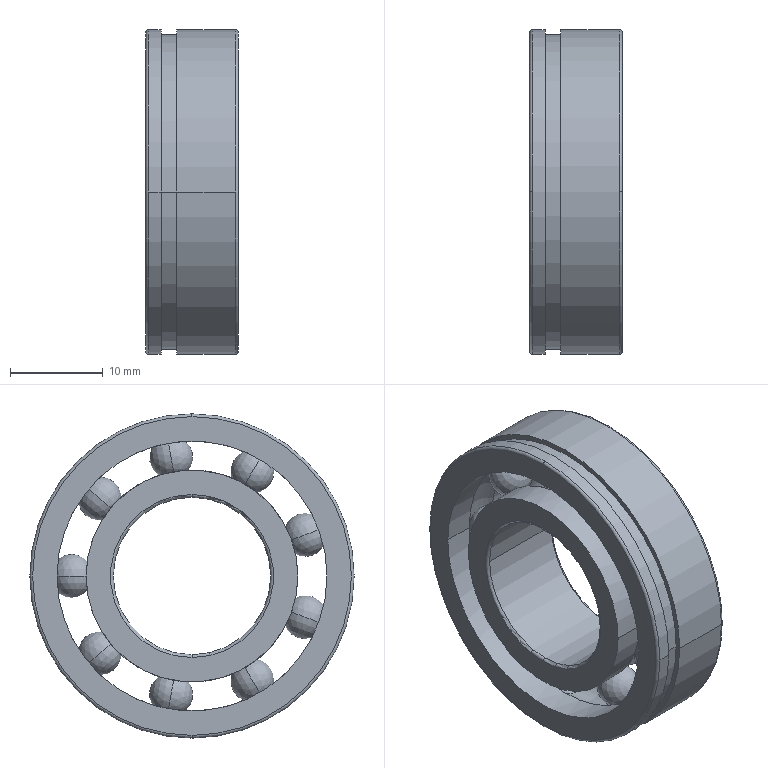Part | SolidWorks | features BaseBody 11 | 11 solids | 54 faces | box 10 x 35 x 35 mm | volume 4868 mm3 | sphere 18 | cylinder 16 | torus 14 | plane 6 | commonest cylinder face diameters 22.868 x4 29.132 x4 35 x4 17 x2 33.92 x2
STEP:
#1=CARTESIAN_POINT('',(5.,10.66,0.));
#2=VERTEX_POINT('',#1);
#3=CARTESIAN_POINT('',(5.,15.34,0.));
#4=VERTEX_POINT('',#3);
#5=CARTESIAN_POINT('',(5.,13.,0.));
#6=DIRECTION('',(0.,0.,1.));
#7=DIRECTION('',(1.,0.,0.));
#8=AXIS2_PLACEMENT_3D('',#5,#6,#7);
#9=CIRCLE('',#8,2.34);
#10=EDGE_CURVE('',#2,#4,#9,.T.);
#11=ORIENTED_EDGE('',*,*,#10,.F.);
#12=CARTESIAN_POINT('',(5.,13.,0.));
#13=DIRECTION('',(0.,0.,-1.));
#14=DIRECTION('',(-1.,0.,0.));
#15=AXIS2_PLACEMENT_3D('',#12,#13,#14);
#16=CIRCLE('',#15,2.34);
#17=EDGE_CURVE('',#2,#4,#16,.T.);
#18=ORIENTED_EDGE('',*,*,#17,.T.);
#19=EDGE_LOOP('',(#11,#18));
#20=FACE_OUTER_BOUND('',#19,.T.);
#21=CARTESIAN_POINT('',(5.,13.,0.));
#22=DIRECTION('',(0.,0.,-1.));
#23=DIRECTION('',(1.,0.,0.));
#24=AXIS2_PLACEMENT_3D('',#21,#22,#23);
#25=SPHERICAL_SURFACE('',#24,2.34);
#26=ADVANCED_FACE('',(#20),#25,.T.);
#27=ORIENTED_EDGE('',*,*,#17,.F.);
#28=ORIENTED_EDGE('',*,*,#10,.T.);
#29=EDGE_LOOP('',(#27,#28));
#30=FACE_OUTER_BOUND('',#29,.T.);
#31=CARTESIAN_POINT('',(5.,13.,0.));
#32=DIRECTION('',(0.,0.,-1.));
#33=DIRECTION('',(1.,0.,0.));
#34=AXIS2_PLACEMENT_3D('',#31,#32,#33);
#35=SPHERICAL_SURFACE('',#34,2.34);
#36=ADVANCED_FACE('',(#30),#35,.T.);
#37=CLOSED_SHELL('',(#26,#36));
#38=MANIFOLD_SOLID_BREP('',#37);
#39=CARTESIAN_POINT('',(3.333,-16.96,0.));
#40=VERTEX_POINT('',#39);
#41=CARTESIAN_POINT('',(3.333,16.96,0.));
#42=VERTEX_POINT('',#41);
#43=CARTESIAN_POINT('',(3.333,0.,0.));
#44=DIRECTION('',(1.,0.,0.));
#45=DIRECTION('',(0.,1.,0.));
#46=AXIS2_PLACEMENT_3D('',#43,#44,#45);
#47=CIRCLE('',#46,16.96);
#48=EDGE_CURVE('',#40,#42,#47,.T.);
#49=ORIENTED_EDGE('',*,*,#48,.F.);
#50=CARTESIAN_POINT('',(1.667,-16.96,0.));
#51=VERTEX_POINT('',#50);
#52=CARTESIAN_POINT('',(2.5,-16.96,0.));
#53=DIRECTION('',(-1.,0.,0.));
#54=VECTOR('',#53,1000.);
#55=LINE('',#52,#54);
#56=EDGE_CURVE('',#40,#51,#55,.T.);
#57=ORIENTED_EDGE('',*,*,#56,.T.);
#58=CARTESIAN_POINT('',(1.667,16.96,0.));
#59=VERTEX_POINT('',#58);
#60=CARTESIAN_POINT('',(1.667,0.,0.));
#61=DIRECTION('',(1.,0.,0.));
#62=DIRECTION('',(0.,1.,0.));
#63=AXIS2_PLACEMENT_3D('',#60,#61,#62);
#64=CIRCLE('',#63,16.96);
#65=EDGE_CURVE('',#51,#59,#64,.T.);
#66=ORIENTED_EDGE('',*,*,#65,.T.);
#67=CARTESIAN_POINT('',(2.5,16.96,0.));
#68=DIRECTION('',(-1.,0.,0.));
#69=VECTOR('',#68,1000.);
#70=LINE('',#67,#69);
#71=EDGE_CURVE('',#42,#59,#70,.T.);
#72=ORIENTED_EDGE('',*,*,#71,.F.);
#73=EDGE_LOOP('',(#49,#57,#66,#72));
#74=FACE_OUTER_BOUND('',#73,.T.);
#75=CARTESIAN_POINT('',(2.5,0.,0.));
#76=DIRECTION('',(-1.,0.,0.));
#77=DIRECTION('',(0.,1.,0.));
#78=AXIS2_PLACEMENT_3D('',#75,#76,#77);
#79=CYLINDRICAL_SURFACE('',#78,16.96);
#80=ADVANCED_FACE('',(#74),#79,.T.);
#81=CARTESIAN_POINT('',(9.7,-17.5,0.));
#82=VERTEX_POINT('',#81);
#83=CARTESIAN_POINT('',(9.7,0.,-17.5));
#84=VERTEX_POINT('',#83);
#85=CARTESIAN_POINT('',(9.7,0.,0.));
#86=DIRECTION('',(1.,0.,0.));
#87=DIRECTION('',(0.,-1.,0.));
#88=AXIS2_PLACEMENT_3D('',#85,#86,#87);
#89=CIRCLE('',#88,17.5);
#90=EDGE_CURVE('',#82,#84,#89,.T.);
#91=ORIENTED_EDGE('',*,*,#90,.F.);
#92=CARTESIAN_POINT('',(3.333,-17.5,0.));
#93=VERTEX_POINT('',#92);
#94=CARTESIAN_POINT('',(6.667,-17.5,0.));
#95=DIRECTION('',(-1.,0.,0.));
#96=VECTOR('',#95,1000.);
#97=LINE('',#94,#96);
#98=EDGE_CURVE('',#82,#93,#97,.T.);
#99=ORIENTED_EDGE('',*,*,#98,.T.);
#100=CARTESIAN_POINT('',(3.333,17.5,0.));
#101=VERTEX_POINT('',#100);
#102=CARTESIAN_POINT('',(3.333,0.,0.));
#103=DIRECTION('',(1.,0.,0.));
#104=DIRECTION('',(0.,1.,0.));
#105=AXIS2_PLACEMENT_3D('',#102,#103,#104);
#106=CIRCLE('',#105,17.5);
#107=EDGE_CURVE('',#93,#101,#106,.T.);
#108=ORIENTED_EDGE('',*,*,#107,.T.);
#109=CARTESIAN_POINT('',(9.7,17.5,0.));
#110=VERTEX_POINT('',#109);
#111=CARTESIAN_POINT('',(6.667,17.5,0.));
#112=DIRECTION('',(-1.,0.,0.));
#113=VECTOR('',#112,1000.);
#114=LINE('',#111,#113);
#115=EDGE_CURVE('',#110,#101,#114,.T.);
#116=ORIENTED_EDGE('',*,*,#115,.F.);
#117=CARTESIAN_POINT('',(9.7,0.,0.));
#118=DIRECTION('',(1.,0.,0.));
#119=DIRECTION('',(0.,-1.,0.));
#120=AXIS2_PLACEMENT_3D('',#117,#118,#119);
#121=CIRCLE('',#120,17.5);
#122=EDGE_CURVE('',#84,#110,#121,.T.);
#123=ORIENTED_EDGE('',*,*,#122,.F.);
#124=EDGE_LOOP('',(#91,#99,#108,#116,#123));
#125=FACE_OUTER_BOUND('',#124,.T.);
#126=CARTESIAN_POINT('',(6.667,0.,0.));
#127=DIRECTION('',(-1.,0.,0.));
#128=DIRECTION('',(0.,1.,0.));
#129=AXIS2_PLACEMENT_3D('',#126,#127,#128);
#130=CYLINDRICAL_SURFACE('',#129,17.5);
#131=ADVANCED_FACE('',(#125),#130,.T.);
#132=CARTESIAN_POINT('',(1.667,-17.5,0.));
#133=VERTEX_POINT('',#132);
#134=CARTESIAN_POINT('',(1.667,17.5,0.));
#135=VERTEX_POINT('',#134);
#136=CARTESIAN_POINT('',(1.667,0.,0.));
#137=DIRECTION('',(1.,0.,0.));
#138=DIRECTION('',(0.,1.,0.));
#139=AXIS2_PLACEMENT_3D('',#136,#137,#138);
#140=CIRCLE('',#139,17.5);
#141=EDGE_CURVE('',#133,#135,#140,.T.);
#142=ORIENTED_EDGE('',*,*,#141,.F.);
#143=CARTESIAN_POINT('',(0.3,-17.5,0.));
#144=VERTEX_POINT('',#143);
#145=CARTESIAN_POINT('',(0.8333,-17.5,0.));
#146=DIRECTION('',(-1.,0.,0.));
#147=VECTOR('',#146,1000.);
#148=LINE('',#145,#147);
#149=EDGE_CURVE('',#133,#144,#148,.T.);
#150=ORIENTED_EDGE('',*,*,#149,.T.);
#151=CARTESIAN_POINT('',(0.3,0.,-17.5));
#152=VERTEX_POINT('',#151);
#153=CARTESIAN_POINT('',(0.3,0.,0.));
#154=DIRECTION('',(-1.,0.,0.));
#155=DIRECTION('',(0.,-1.,0.));
#156=AXIS2_PLACEMENT_3D('',#153,#154,#155);
#157=CIRCLE('',#156,17.5);
#158=EDGE_CURVE('',#152,#144,#157,.T.);
#159=ORIENTED_EDGE('',*,*,#158,.F.);
#160=CARTESIAN_POINT('',(0.3,17.5,0.));
#161=VERTEX_POINT('',#160);
#162=CARTESIAN_POINT('',(0.3,0.,0.));
#163=DIRECTION('',(-1.,0.,0.));
#164=DIRECTION('',(0.,-1.,0.));
#165=AXIS2_PLACEMENT_3D('',#162,#163,#164);
#166=CIRCLE('',#165,17.5);
#167=EDGE_CURVE('',#161,#152,#166,.T.);
#168=ORIENTED_EDGE('',*,*,#167,.F.);
#169=CARTESIAN_POINT('',(0.8333,17.5,0.));
#170=DIRECTION('',(-1.,0.,0.));
#171=VECTOR('',#170,1000.);
#172=LINE('',#169,#171);
#173=EDGE_CURVE('',#135,#161,#172,.T.);
#174=ORIENTED_EDGE('',*,*,#173,.F.);
#175=EDGE_LOOP('',(#142,#150,#159,#168,#174));
#176=FACE_OUTER_BOUND('',#175,.T.);
#177=CARTESIAN_POINT('',(0.8333,0.,0.));
#178=DIRECTION('',(-1.,0.,0.));
#179=DIRECTION('',(0.,1.,0.));
#180=AXIS2_PLACEMENT_3D('',#177,#178,#179);
#181=CYLINDRICAL_SURFACE('',#180,17.5);
#182=ADVANCED_FACE('',(#176),#181,.T.);
#183=ORIENTED_EDGE('',*,*,#122,.T.);
#184=CARTESIAN_POINT('',(9.7,0.,17.5));
#185=VERTEX_POINT('',#184);
#186=CARTESIAN_POINT('',(9.7,0.,0.));
#187=DIRECTION('',(1.,0.,0.));
#188=DIRECTION('',(0.,-1.,0.));
#189=AXIS2_PLACEMENT_3D('',#186,#187,#188);
#190=CIRCLE('',#189,17.5);
#191=EDGE_CURVE('',#110,#185,#190,.T.);
#192=ORIENTED_EDGE('',*,*,#191,.T.);
#193=CARTESIAN_POINT('',(10.,0.,17.2));
#194=VERTEX_POINT('',#193);
#195=CARTESIAN_POINT('',(9.7,0.,17.2));
#196=DIRECTION('',(0.,1.,0.));
#197=DIRECTION('',(0.,0.,1.));
#198=AXIS2_PLACEMENT_3D('',#195,#196,#197);
#199=CIRCLE('',#198,0.3);
#200=EDGE_CURVE('',#185,#194,#199,.T.);
#201=ORIENTED_EDGE('',*,*,#200,.T.);
#202=CARTESIAN_POINT('',(10.,0.,-17.2));
#203=VERTEX_POINT('',#202);
#204=CARTESIAN_POINT('',(10.,0.,0.));
#205=DIRECTION('',(-1.,0.,0.));
#206=DIRECTION('',(0.,-1.,0.));
#207=AXIS2_PLACEMENT_3D('',#204,#205,#206);
#208=CIRCLE('',#207,17.2);
#209=EDGE_CURVE('',#194,#203,#208,.T.);
#210=ORIENTED_EDGE('',*,*,#209,.T.);
#211=CARTESIAN_POINT('',(9.7,0.,-17.2));
#212=DIRECTION('',(0.,-1.,0.));
#213=DIRECTION('',(0.,0.,-1.));
#214=AXIS2_PLACEMENT_3D('',#211,#212,#213);
#215=CIRCLE('',#214,0.3);
#216=EDGE_CURVE('',#84,#203,#215,.T.);
#217=ORIENTED_EDGE('',*,*,#216,.F.);
#218=EDGE_LOOP('',(#183,#192,#201,#210,#217));
#219=FACE_OUTER_BOUND('',#218,.T.);
#220=CARTESIAN_POINT('',(9.7,0.,0.));
#221=DIRECTION('',(1.,0.,0.));
#222=DIRECTION('',(0.,0.,-1.));
#223=AXIS2_PLACEMENT_3D('',#220,#221,#222);
#224=TOROIDAL_SURFACE('',#223,17.2,0.3);
#225=ADVANCED_FACE('',(#219),#224,.T.);
#226=CARTESIAN_POINT('',(0.,0.,-17.2));
#227=VERTEX_POINT('',#226);
#228=CARTESIAN_POINT('',(0.,0.,17.2));
#229=VERTEX_POINT('',#228);
#230=CARTESIAN_POINT('',(0.,0.,0.));
#231=DIRECTION('',(1.,0.,0.));
#232=DIRECTION('',(0.,-1.,0.));
#233=AXIS2_PLACEMENT_3D('',#230,#231,#232);
#234=CIRCLE('',#233,17.2);
#235=EDGE_CURVE('',#227,#229,#234,.T.);
#236=ORIENTED_EDGE('',*,*,#235,.T.);
#237=CARTESIAN_POINT('',(0.3,0.,17.5));
#238=VERTEX_POINT('',#237);
#239=CARTESIAN_POINT('',(0.3,0.,17.2));
#240=DIRECTION('',(0.,1.,0.));
#241=DIRECTION('',(0.,0.,1.));
#242=AXIS2_PLACEMENT_3D('',#239,#240,#241);
#243=CIRCLE('',#242,0.3);
#244=EDGE_CURVE('',#229,#238,#243,.T.);
#245=ORIENTED_EDGE('',*,*,#244,.T.);
#246=CARTESIAN_POINT('',(0.3,0.,0.));
#247=DIRECTION('',(-1.,0.,0.));
#248=DIRECTION('',(0.,-1.,0.));
#249=AXIS2_PLACEMENT_3D('',#246,#247,#248);
#250=CIRCLE('',#249,17.5);
#251=EDGE_CURVE('',#238,#161,#250,.T.);
#252=ORIENTED_EDGE('',*,*,#251,.T.);
#253=ORIENTED_EDGE('',*,*,#167,.T.);
#254=CARTESIAN_POINT('',(0.3,0.,-17.2));
#255=DIRECTION('',(0.,-1.,0.));
#256=DIRECTION('',(0.,0.,-1.));
#257=AXIS2_PLACEMENT_3D('',#254,#255,#256);
#258=CIRCLE('',#257,0.3);
#259=EDGE_CURVE('',#227,#152,#258,.T.);
#260=ORIENTED_EDGE('',*,*,#259,.F.);
#261=EDGE_LOOP('',(#236,#245,#252,#253,#260));
#262=FACE_OUTER_BOUND('',#261,.T.);
#263=CARTESIAN_POINT('',(0.3,0.,0.));
#264=DIRECTION('',(1.,0.,0.));
#265=DIRECTION('',(0.,0.,-1.));
#266=AXIS2_PLACEMENT_3D('',#263,#264,#265);
#267=TOROIDAL_SURFACE('',#266,17.2,0.3);
#268=ADVANCED_FACE('',(#262),#267,.T.);
#269=CARTESIAN_POINT('',(3.261,0.,14.566));
#270=VERTEX_POINT('',#269);
#271=CARTESIAN_POINT('',(3.261,-14.566,0.));
#272=VERTEX_POINT('',#271);
#273=CARTESIAN_POINT('',(3.261,0.,0.));
#274=DIRECTION('',(1.,0.,0.));
#275=DIRECTION('',(0.,1.,0.));
#276=AXIS2_PLACEMENT_3D('',#273,#274,#275);
#277=CIRCLE('',#276,14.566);
#278=EDGE_CURVE('',#270,#272,#277,.T.);
#279=ORIENTED_EDGE('',*,*,#278,.F.);
#280=CARTESIAN_POINT('',(6.739,0.,14.566));
#281=VERTEX_POINT('',#280);
#282=CARTESIAN_POINT('',(5.,0.,13.));
#283=DIRECTION('',(0.,1.,0.));
#284=DIRECTION('',(0.,0.,1.));
#285=AXIS2_PLACEMENT_3D('',#282,#283,#284);
#286=CIRCLE('',#285,2.34);
#287=EDGE_CURVE('',#270,#281,#286,.T.);
#288=ORIENTED_EDGE('',*,*,#287,.T.);
#289=CARTESIAN_POINT('',(6.739,-14.566,0.));
#290=VERTEX_POINT('',#289);
#291=CARTESIAN_POINT('',(6.739,0.,0.));
#292=DIRECTION('',(1.,0.,0.));
#293=DIRECTION('',(0.,1.,0.));
#294=AXIS2_PLACEMENT_3D('',#291,#292,#293);
#295=CIRCLE('',#294,14.566);
#296=EDGE_CURVE('',#281,#290,#295,.T.);
#297=ORIENTED_EDGE('',*,*,#296,.T.);
#298=CARTESIAN_POINT('',(6.739,0.,-14.566));
#299=VERTEX_POINT('',#298);
#300=CARTESIAN_POINT('',(6.739,0.,0.));
#301=DIRECTION('',(1.,0.,0.));
#302=DIRECTION('',(0.,1.,0.));
#303=AXIS2_PLACEMENT_3D('',#300,#301,#302);
#304=CIRCLE('',#303,14.566);
#305=EDGE_CURVE('',#290,#299,#304,.T.);
#306=ORIENTED_EDGE('',*,*,#305,.T.);
#307=CARTESIAN_POINT('',(3.261,0.,-14.566));
#308=VERTEX_POINT('',#307);
#309=CARTESIAN_POINT('',(5.,0.,-13.));
#310=DIRECTION('',(0.,-1.,0.));
#311=DIRECTION('',(0.,0.,-1.));
#312=AXIS2_PLACEMENT_3D('',#309,#310,#311);
#313=CIRCLE('',#312,2.34);
#314=EDGE_CURVE('',#308,#299,#313,.T.);
#315=ORIENTED_EDGE('',*,*,#314,.F.);
#316=CARTESIAN_POINT('',(3.261,0.,0.));
#317=DIRECTION('',(1.,0.,0.));
#318=DIRECTION('',(0.,1.,0.));
#319=AXIS2_PLACEMENT_3D('',#316,#317,#318);
#320=CIRCLE('',#319,14.566);
#321=EDGE_CURVE('',#272,#308,#320,.T.);
#322=ORIENTED_EDGE('',*,*,#321,.F.);
#323=EDGE_LOOP('',(#279,#288,#297,#306,#315,#322));
#324=FACE_OUTER_BOUND('',#323,.T.);
#325=CARTESIAN_POINT('',(5.,0.,0.));
#326=DIRECTION('',(1.,0.,0.));
#327=DIRECTION('',(0.,0.,-1.));
#328=AXIS2_PLACEMENT_3D('',#325,#326,#327);
#329=TOROIDAL_SURFACE('',#328,13.,2.34);
#330=ADVANCED_FACE('',(#324),#329,.F.);
#331=CARTESIAN_POINT('',(10.,14.566,0.));
#332=VERTEX_POINT('',#331);
#333=CARTESIAN_POINT('',(10.,-14.566,0.));
#334=VERTEX_POINT('',#333);
#335=CARTESIAN_POINT('',(10.,0.,0.));
#336=DIRECTION('',(1.,0.,0.));
#337=DIRECTION('',(0.,1.,0.));
#338=AXIS2_PLACEMENT_3D('',#335,#336,#337);
#339=CIRCLE('',#338,14.566);
#340=EDGE_CURVE('',#332,#334,#339,.T.);
#341=ORIENTED_EDGE('',*,*,#340,.T.);
#342=CARTESIAN_POINT('',(8.369,-14.566,0.));
#343=DIRECTION('',(-1.,0.,0.));
#344=VECTOR('',#343,1000.);
#345=LINE('',#342,#344);
#346=EDGE_CURVE('',#334,#290,#345,.T.);
#347=ORIENTED_EDGE('',*,*,#346,.T.);
#348=ORIENTED_EDGE('',*,*,#296,.F.);
#349=CARTESIAN_POINT('',(6.739,14.566,0.));
#350=VERTEX_POINT('',#349);
#351=CARTESIAN_POINT('',(6.739,0.,0.));
#352=DIRECTION('',(1.,0.,0.));
#353=DIRECTION('',(0.,1.,0.));
#354=AXIS2_PLACEMENT_3D('',#351,#352,#353);
#355=CIRCLE('',#354,14.566);
#356=EDGE_CURVE('',#350,#281,#355,.T.);
#357=ORIENTED_EDGE('',*,*,#356,.F.);
#358=CARTESIAN_POINT('',(8.369,14.566,0.));
#359=DIRECTION('',(-1.,0.,0.));
#360=VECTOR('',#359,1000.);
#361=LINE('',#358,#360);
#362=EDGE_CURVE('',#332,#350,#361,.T.);
#363=ORIENTED_EDGE('',*,*,#362,.F.);
#364=EDGE_LOOP('',(#341,#347,#348,#357,#363));
#365=FACE_OUTER_BOUND('',#364,.T.);
#366=CARTESIAN_POINT('',(8.369,0.,0.));
#367=DIRECTION('',(-1.,0.,0.));
#368=DIRECTION('',(0.,1.,0.));
#369=AXIS2_PLACEMENT_3D('',#366,#367,#368);
#370=CYLINDRICAL_SURFACE('',#369,14.566);
#371=ADVANCED_FACE('',(#365),#370,.F.);
#372=CARTESIAN_POINT('',(3.261,14.566,0.));
#373=VERTEX_POINT('',#372);
#374=CARTESIAN_POINT('',(3.261,0.,0.));
#375=DIRECTION('',(1.,0.,0.));
#376=DIRECTION('',(0.,1.,0.));
#377=AXIS2_PLACEMENT_3D('',#374,#375,#376);
#378=CIRCLE('',#377,14.566);
#379=EDGE_CURVE('',#373,#270,#378,.T.);
#380=ORIENTED_EDGE('',*,*,#379,.T.);
#381=ORIENTED_EDGE('',*,*,#278,.T.);
#382=CARTESIAN_POINT('',(0.,-14.566,0.));
#383=VERTEX_POINT('',#382);
#384=CARTESIAN_POINT('',(1.631,-14.566,0.));
#385=DIRECTION('',(-1.,0.,0.));
#386=VECTOR('',#385,1000.);
#387=LINE('',#384,#386);
#388=EDGE_CURVE('',#272,#383,#387,.T.);
#389=ORIENTED_EDGE('',*,*,#388,.T.);
#390=CARTESIAN_POINT('',(0.,14.566,0.));
#391=VERTEX_POINT('',#390);
#392=CARTESIAN_POINT('',(0.,0.,0.));
#393=DIRECTION('',(1.,0.,0.));
#394=DIRECTION('',(0.,1.,0.));
#395=AXIS2_PLACEMENT_3D('',#392,#393,#394);
#396=CIRCLE('',#395,14.566);
#397=EDGE_CURVE('',#391,#383,#396,.T.);
#398=ORIENTED_EDGE('',*,*,#397,.F.);
#399=CARTESIAN_POINT('',(1.631,14.566,0.));
#400=DIRECTION('',(-1.,0.,0.));
#401=VECTOR('',#400,1000.);
#402=LINE('',#399,#401);
#403=EDGE_CURVE('',#373,#391,#402,.T.);
#404=ORIENTED_EDGE('',*,*,#403,.F.);
#405=EDGE_LOOP('',(#380,#381,#389,#398,#404));
#406=FACE_OUTER_BOUND('',#405,.T.);
#407=CARTESIAN_POINT('',(1.631,0.,0.));
#408=DIRECTION('',(-1.,0.,0.));
#409=DIRECTION('',(0.,1.,0.));
#410=AXIS2_PLACEMENT_3D('',#407,#408,#409);
#411=CYLINDRICAL_SURFACE('',#410,14.566);
#412=ADVANCED_FACE('',(#406),#411,.F.);
#413=CARTESIAN_POINT('',(3.333,0.,0.));
#414=DIRECTION('',(1.,0.,0.));
#415=DIRECTION('',(0.,1.,0.));
#416=AXIS2_PLACEMENT_3D('',#413,#414,#415);
#417=CIRCLE('',#416,16.96);
#418=EDGE_CURVE('',#42,#40,#417,.T.);
#419=ORIENTED_EDGE('',*,*,#418,.T.);
#420=ORIENTED_EDGE('',*,*,#48,.T.);
#421=EDGE_LOOP('',(#419,#420));
#422=FACE_BOUND('',#421,.T.);
#423=CARTESIAN_POINT('',(3.333,0.,0.));
#424=DIRECTION('',(1.,0.,0.));
#425=DIRECTION('',(0.,1.,0.));
#426=AXIS2_PLACEMENT_3D('',#423,#424,#425);
#427=CIRCLE('',#426,17.5);
#428=EDGE_CURVE('',#101,#93,#427,.T.);
#429=ORIENTED_EDGE('',*,*,#428,.F.);
#430=ORIENTED_EDGE('',*,*,#107,.F.);
#431=EDGE_LOOP('',(#429,#430));
#432=FACE_OUTER_BOUND('',#431,.T.);
#433=CARTESIAN_POINT('',(3.333,17.23,0.));
#434=DIRECTION('',(-1.,0.,0.));
#435=DIRECTION('',(0.,0.,1.));
#436=AXIS2_PLACEMENT_3D('',#433,#434,#435);
#437=PLANE('',#436);
#438=ADVANCED_FACE('',(#422,#432),#437,.T.);
#439=CARTESIAN_POINT('',(1.667,0.,0.));
#440=DIRECTION('',(1.,0.,0.));
#441=DIRECTION('',(0.,1.,0.));
#442=AXIS2_PLACEMENT_3D('',#439,#440,#441);
#443=CIRCLE('',#442,16.96);
#444=EDGE_CURVE('',#59,#51,#443,.T.);
#445=ORIENTED_EDGE('',*,*,#444,.F.);
#446=ORIENTED_EDGE('',*,*,#65,.F.);
#447=EDGE_LOOP('',(#445,#446));
#448=FACE_BOUND('',#447,.T.);
#449=CARTESIAN_POINT('',(1.667,0.,0.));
#450=DIRECTION('',(1.,0.,0.));
#451=DIRECTION('',(0.,1.,0.));
#452=AXIS2_PLACEMENT_3D('',#449,#450,#451);
#453=CIRCLE('',#452,17.5);
#454=EDGE_CURVE('',#135,#133,#453,.T.);
#455=ORIENTED_EDGE('',*,*,#454,.T.);
#456=ORIENTED_EDGE('',*,*,#141,.T.);
#457=EDGE_LOOP('',(#455,#456));
#458=FACE_OUTER_BOUND('',#457,.T.);
#459=CARTESIAN_POINT('',(1.667,17.23,0.));
#460=DIRECTION('',(1.,0.,0.));
#461=DIRECTION('',(0.,1.,0.));
#462=AXIS2_PLACEMENT_3D('',#459,#460,#461);
#463=PLANE('',#462);
#464=ADVANCED_FACE('',(#448,#458),#463,.T.);
#465=ORIENTED_EDGE('',*,*,#340,.F.);
#466=CARTESIAN_POINT('',(10.,0.,0.));
#467=DIRECTION('',(1.,0.,0.));
#468=DIRECTION('',(0.,1.,0.));
#469=AXIS2_PLACEMENT_3D('',#466,#467,#468);
#470=CIRCLE('',#469,14.566);
#471=EDGE_CURVE('',#334,#332,#470,.T.);
#472=ORIENTED_EDGE('',*,*,#471,.F.);
#473=EDGE_LOOP('',(#465,#472));
#474=FACE_BOUND('',#473,.T.);
#475=CARTESIAN_POINT('',(10.,0.,0.));
#476=DIRECTION('',(-1.,0.,0.));
#477=DIRECTION('',(0.,-1.,0.));
#478=AXIS2_PLACEMENT_3D('',#475,#476,#477);
#479=CIRCLE('',#478,17.2);
#480=EDGE_CURVE('',#203,#194,#479,.T.);
#481=ORIENTED_EDGE('',*,*,#480,.F.);
#482=ORIENTED_EDGE('',*,*,#209,.F.);
#483=EDGE_LOOP('',(#481,#482));
#484=FACE_OUTER_BOUND('',#483,.T.);
#485=CARTESIAN_POINT('',(10.,16.033,0.));
#486=DIRECTION('',(1.,0.,0.));
#487=DIRECTION('',(0.,1.,0.));
#488=AXIS2_PLACEMENT_3D('',#485,#486,#487);
#489=PLANE('',#488);
#490=ADVANCED_FACE('',(#474,#484),#489,.T.);
#491=ORIENTED_EDGE('',*,*,#397,.T.);
#492=CARTESIAN_POINT('',(0.,0.,0.));
#493=DIRECTION('',(1.,0.,0.));
#494=DIRECTION('',(0.,1.,0.));
#495=AXIS2_PLACEMENT_3D('',#492,#493,#494);
#496=CIRCLE('',#495,14.566);
#497=EDGE_CURVE('',#383,#391,#496,.T.);
#498=ORIENTED_EDGE('',*,*,#497,.T.);
#499=EDGE_LOOP('',(#491,#498));
#500=FACE_BOUND('',#499,.T.);
#501=ORIENTED_EDGE('',*,*,#235,.F.);
#502=CARTESIAN_POINT('',(0.,0.,0.));
#503=DIRECTION('',(1.,0.,0.));
#504=DIRECTION('',(0.,-1.,0.));
#505=AXIS2_PLACEMENT_3D('',#502,#503,#504);
#506=CIRCLE('',#505,17.2);
#507=EDGE_CURVE('',#229,#227,#506,.T.);
#508=ORIENTED_EDGE('',*,*,#507,.F.);
#509=EDGE_LOOP('',(#501,#508));
#510=FACE_OUTER_BOUND('',#509,.T.);
#511=CARTESIAN_POINT('',(0.,16.033,0.));
#512=DIRECTION('',(-1.,0.,0.));
#513=DIRECTION('',(0.,0.,1.));
#514=AXIS2_PLACEMENT_3D('',#511,#512,#513);
#515=PLANE('',#514);
#516=ADVANCED_FACE('',(#500,#510),#515,.T.);
#517=ORIENTED_EDGE('',*,*,#388,.F.);
#518=ORIENTED_EDGE('',*,*,#321,.T.);
#519=CARTESIAN_POINT('',(3.261,0.,0.));
#520=DIRECTION('',(1.,0.,0.));
#521=DIRECTION('',(0.,1.,0.));
#522=AXIS2_PLACEMENT_3D('',#519,#520,#521);
#523=CIRCLE('',#522,14.566);
#524=EDGE_CURVE('',#308,#373,#523,.T.);
#525=ORIENTED_EDGE('',*,*,#524,.T.);
#526=ORIENTED_EDGE('',*,*,#403,.T.);
#527=ORIENTED_EDGE('',*,*,#497,.F.);
#528=EDGE_LOOP('',(#517,#518,#525,#526,#527));
#529=FACE_OUTER_BOUND('',#528,.T.);
#530=CARTESIAN_POINT('',(1.631,0.,0.));
#531=DIRECTION('',(-1.,0.,0.));
#532=DIRECTION('',(0.,1.,0.));
#533=AXIS2_PLACEMENT_3D('',#530,#531,#532);
#534=CYLINDRICAL_SURFACE('',#533,14.566);
#535=ADVANCED_FACE('',(#529),#534,.F.);
#536=ORIENTED_EDGE('',*,*,#346,.F.);
#537=ORIENTED_EDGE('',*,*,#471,.T.);
#538=ORIENTED_EDGE('',*,*,#362,.T.);
#539=CARTESIAN_POINT('',(6.739,0.,0.));
#540=DIRECTION('',(1.,0.,0.));
#541=DIRECTION('',(0.,1.,0.));
#542=AXIS2_PLACEMENT_3D('',#539,#540,#541);
#543=CIRCLE('',#542,14.566);
#544=EDGE_CURVE('',#299,#350,#543,.T.);
#545=ORIENTED_EDGE('',*,*,#544,.F.);
#546=ORIENTED_EDGE('',*,*,#305,.F.);
#547=EDGE_LOOP('',(#536,#537,#538,#545,#546));
#548=FACE_OUTER_BOUND('',#547,.T.);
#549=CARTESIAN_POINT('',(8.369,0.,0.));
#550=DIRECTION('',(-1.,0.,0.));
#551=DIRECTION('',(0.,1.,0.));
#552=AXIS2_PLACEMENT_3D('',#549,#550,#551);
#553=CYLINDRICAL_SURFACE('',#552,14.566);
#554=ADVANCED_FACE('',(#548),#553,.F.);
#555=ORIENTED_EDGE('',*,*,#287,.F.);
#556=ORIENTED_EDGE('',*,*,#379,.F.);
#557=ORIENTED_EDGE('',*,*,#524,.F.);
#558=ORIENTED_EDGE('',*,*,#314,.T.);
#559=ORIENTED_EDGE('',*,*,#544,.T.);
#560=ORIENTED_EDGE('',*,*,#356,.T.);
#561=EDGE_LOOP('',(#555,#556,#557,#558,#559,#560));
#562=FACE_OUTER_BOUND('',#561,.T.);
#563=CARTESIAN_POINT('',(5.,0.,0.));
#564=DIRECTION('',(1.,0.,0.));
#565=DIRECTION('',(0.,0.,-1.));
#566=AXIS2_PLACEMENT_3D('',#563,#564,#565);
#567=TOROIDAL_SURFACE('',#566,13.,2.34);
#568=ADVANCED_FACE('',(#562),#567,.F.);
#569=ORIENTED_EDGE('',*,*,#244,.F.);
#570=ORIENTED_EDGE('',*,*,#507,.T.);
#571=ORIENTED_EDGE('',*,*,#259,.T.);
#572=ORIENTED_EDGE('',*,*,#158,.T.);
#573=CARTESIAN_POINT('',(0.3,0.,0.));
#574=DIRECTION('',(-1.,0.,0.));
#575=DIRECTION('',(0.,-1.,0.));
#576=AXIS2_PLACEMENT_3D('',#573,#574,#575);
#577=CIRCLE('',#576,17.5);
#578=EDGE_CURVE('',#144,#238,#577,.T.);
#579=ORIENTED_EDGE('',*,*,#578,.T.);
#580=EDGE_LOOP('',(#569,#570,#571,#572,#579));
#581=FACE_OUTER_BOUND('',#580,.T.);
#582=CARTESIAN_POINT('',(0.3,0.,0.));
#583=DIRECTION('',(1.,0.,0.));
#584=DIRECTION('',(0.,0.,-1.));
#585=AXIS2_PLACEMENT_3D('',#582,#583,#584);
#586=TOROIDAL_SURFACE('',#585,17.2,0.3);
#587=ADVANCED_FACE('',(#581),#586,.T.);
#588=ORIENTED_EDGE('',*,*,#200,.F.);
#589=CARTESIAN_POINT('',(9.7,0.,0.));
#590=DIRECTION('',(1.,0.,0.));
#591=DIRECTION('',(0.,-1.,0.));
#592=AXIS2_PLACEMENT_3D('',#589,#590,#591);
#593=CIRCLE('',#592,17.5);
#594=EDGE_CURVE('',#185,#82,#593,.T.);
#595=ORIENTED_EDGE('',*,*,#594,.T.);
#596=ORIENTED_EDGE('',*,*,#90,.T.);
#597=ORIENTED_EDGE('',*,*,#216,.T.);
#598=ORIENTED_EDGE('',*,*,#480,.T.);
#599=EDGE_LOOP('',(#588,#595,#596,#597,#598));
#600=FACE_OUTER_BOUND('',#599,.T.);
#601=CARTESIAN_POINT('',(9.7,0.,0.));
#602=DIRECTION('',(1.,0.,0.));
#603=DIRECTION('',(0.,0.,-1.));
#604=AXIS2_PLACEMENT_3D('',#601,#602,#603);
#605=TOROIDAL_SURFACE('',#604,17.2,0.3);
#606=ADVANCED_FACE('',(#600),#605,.T.);
#607=ORIENTED_EDGE('',*,*,#149,.F.);
#608=ORIENTED_EDGE('',*,*,#454,.F.);
#609=ORIENTED_EDGE('',*,*,#173,.T.);
#610=ORIENTED_EDGE('',*,*,#251,.F.);
#611=ORIENTED_EDGE('',*,*,#578,.F.);
#612=EDGE_LOOP('',(#607,#608,#609,#610,#611));
#613=FACE_OUTER_BOUND('',#612,.T.);
#614=CARTESIAN_POINT('',(0.8333,0.,0.));
#615=DIRECTION('',(-1.,0.,0.));
#616=DIRECTION('',(0.,1.,0.));
#617=AXIS2_PLACEMENT_3D('',#614,#615,#616);
#618=CYLINDRICAL_SURFACE('',#617,17.5);
#619=ADVANCED_FACE('',(#613),#618,.T.);
#620=ORIENTED_EDGE('',*,*,#98,.F.);
#621=ORIENTED_EDGE('',*,*,#594,.F.);
#622=ORIENTED_EDGE('',*,*,#191,.F.);
#623=ORIENTED_EDGE('',*,*,#115,.T.);
#624=ORIENTED_EDGE('',*,*,#428,.T.);
#625=EDGE_LOOP('',(#620,#621,#622,#623,#624));
#626=FACE_OUTER_BOUND('',#625,.T.);
#627=CARTESIAN_POINT('',(6.667,0.,0.));
#628=DIRECTION('',(-1.,0.,0.));
#629=DIRECTION('',(0.,1.,0.));
#630=AXIS2_PLACEMENT_3D('',#627,#628,#629);
#631=CYLINDRICAL_SURFACE('',#630,17.5);
#632=ADVANCED_FACE('',(#626),#631,.T.);
#633=ORIENTED_EDGE('',*,*,#56,.F.);
#634=ORIENTED_EDGE('',*,*,#418,.F.);
#635=ORIENTED_EDGE('',*,*,#71,.T.);
#636=ORIENTED_EDGE('',*,*,#444,.T.);
#637=EDGE_LOOP('',(#633,#634,#635,#636));
#638=FACE_OUTER_BOUND('',#637,.T.);
#639=CARTESIAN_POINT('',(2.5,0.,0.));
#640=DIRECTION('',(-1.,0.,0.));
#641=DIRECTION('',(0.,1.,0.));
#642=AXIS2_PLACEMENT_3D('',#639,#640,#641);
#643=CYLINDRICAL_SURFACE('',#642,16.96);
#644=ADVANCED_FACE('',(#638),#643,.T.);
#645=CLOSED_SHELL('',(#80,#131,#182,#225,#268,#330,#371,#412,#438,#464,#490,#516,#535,#554,#568,#587,#606,#619,#632,#644));
#646=MANIFOLD_SOLID_BREP('',#645);
#647=CARTESIAN_POINT('',(6.739,0.,-11.434));
#648=VERTEX_POINT('',#647);
#649=CARTESIAN_POINT('',(5.,0.,-10.66));
#650=VERTEX_POINT('',#649);
#651=CARTESIAN_POINT('',(5.,0.,-13.));
#652=DIRECTION('',(0.,-1.,0.));
#653=DIRECTION('',(0.,0.,-1.));
#654=AXIS2_PLACEMENT_3D('',#651,#652,#653);
#655=CIRCLE('',#654,2.34);
#656=EDGE_CURVE('',#648,#650,#655,.T.);
#657=ORIENTED_EDGE('',*,*,#656,.T.);
#658=CARTESIAN_POINT('',(5.,0.,10.66));
#659=VERTEX_POINT('',#658);
#660=CARTESIAN_POINT('',(5.,0.,0.));
#661=DIRECTION('',(1.,0.,0.));
#662=DIRECTION('',(0.,0.,-1.));
#663=AXIS2_PLACEMENT_3D('',#660,#661,#662);
#664=CIRCLE('',#663,10.66);
#665=EDGE_CURVE('',#650,#659,#664,.T.);
#666=ORIENTED_EDGE('',*,*,#665,.T.);
#667=CARTESIAN_POINT('',(6.739,0.,11.434));
#668=VERTEX_POINT('',#667);
#669=CARTESIAN_POINT('',(5.,0.,13.));
#670=DIRECTION('',(0.,1.,0.));
#671=DIRECTION('',(0.,0.,1.));
#672=AXIS2_PLACEMENT_3D('',#669,#670,#671);
#673=CIRCLE('',#672,2.34);
#674=EDGE_CURVE('',#668,#659,#673,.T.);
#675=ORIENTED_EDGE('',*,*,#674,.F.);
#676=CARTESIAN_POINT('',(6.739,11.434,0.));
#677=VERTEX_POINT('',#676);
#678=CARTESIAN_POINT('',(6.739,0.,0.));
#679=DIRECTION('',(1.,0.,0.));
#680=DIRECTION('',(0.,1.,0.));
#681=AXIS2_PLACEMENT_3D('',#678,#679,#680);
#682=CIRCLE('',#681,11.434);
#683=EDGE_CURVE('',#677,#668,#682,.T.);
#684=ORIENTED_EDGE('',*,*,#683,.F.);
#685=CARTESIAN_POINT('',(6.739,0.,0.));
#686=DIRECTION('',(1.,0.,0.));
#687=DIRECTION('',(0.,1.,0.));
#688=AXIS2_PLACEMENT_3D('',#685,#686,#687);
#689=CIRCLE('',#688,11.434);
#690=EDGE_CURVE('',#648,#677,#689,.T.);
#691=ORIENTED_EDGE('',*,*,#690,.F.);
#692=EDGE_LOOP('',(#657,#666,#675,#684,#691));
#693=FACE_OUTER_BOUND('',#692,.T.);
#694=CARTESIAN_POINT('',(5.,0.,0.));
#695=DIRECTION('',(1.,0.,0.));
#696=DIRECTION('',(0.,0.,-1.));
#697=AXIS2_PLACEMENT_3D('',#694,#695,#696);
#698=TOROIDAL_SURFACE('',#697,13.,2.34);
#699=ADVANCED_FACE('',(#693),#698,.F.);
#700=ORIENTED_EDGE('',*,*,#674,.T.);
#701=CARTESIAN_POINT('',(5.,0.,0.));
#702=DIRECTION('',(1.,0.,0.));
#703=DIRECTION('',(0.,0.,-1.));
#704=AXIS2_PLACEMENT_3D('',#701,#702,#703);
#705=CIRCLE('',#704,10.66);
#706=EDGE_CURVE('',#659,#650,#705,.T.);
#707=ORIENTED_EDGE('',*,*,#706,.T.);
#708=ORIENTED_EDGE('',*,*,#656,.F.);
#709=CARTESIAN_POINT('',(6.739,-11.434,0.));
#710=VERTEX_POINT('',#709);
#711=CARTESIAN_POINT('',(6.739,0.,0.));
#712=DIRECTION('',(1.,0.,0.));
#713=DIRECTION('',(0.,1.,0.));
#714=AXIS2_PLACEMENT_3D('',#711,#712,#713);
#715=CIRCLE('',#714,11.434);
#716=EDGE_CURVE('',#710,#648,#715,.T.);
#717=ORIENTED_EDGE('',*,*,#716,.F.);
#718=CARTESIAN_POINT('',(6.739,0.,0.));
#719=DIRECTION('',(1.,0.,0.));
#720=DIRECTION('',(0.,1.,0.));
#721=AXIS2_PLACEMENT_3D('',#718,#719,#720);
#722=CIRCLE('',#721,11.434);
#723=EDGE_CURVE('',#668,#710,#722,.T.);
#724=ORIENTED_EDGE('',*,*,#723,.F.);
#725=EDGE_LOOP('',(#700,#707,#708,#717,#724));
#726=FACE_OUTER_BOUND('',#725,.T.);
#727=CARTESIAN_POINT('',(5.,0.,0.));
#728=DIRECTION('',(1.,0.,0.));
#729=DIRECTION('',(0.,0.,-1.));
#730=AXIS2_PLACEMENT_3D('',#727,#728,#729);
#731=TOROIDAL_SURFACE('',#730,13.,2.34);
#732=ADVANCED_FACE('',(#726),#731,.F.);
#733=ORIENTED_EDGE('',*,*,#706,.F.);
#734=CARTESIAN_POINT('',(3.261,0.,11.434));
#735=VERTEX_POINT('',#734);
#736=CARTESIAN_POINT('',(5.,0.,13.));
#737=DIRECTION('',(0.,1.,0.));
#738=DIRECTION('',(0.,0.,1.));
#739=AXIS2_PLACEMENT_3D('',#736,#737,#738);
#740=CIRCLE('',#739,2.34);
#741=EDGE_CURVE('',#659,#735,#740,.T.);
#742=ORIENTED_EDGE('',*,*,#741,.T.);
#743=CARTESIAN_POINT('',(3.261,-11.434,0.));
#744=VERTEX_POINT('',#743);
#745=CARTESIAN_POINT('',(3.261,0.,0.));
#746=DIRECTION('',(1.,0.,0.));
#747=DIRECTION('',(0.,1.,0.));
#748=AXIS2_PLACEMENT_3D('',#745,#746,#747);
#749=CIRCLE('',#748,11.434);
#750=EDGE_CURVE('',#735,#744,#749,.T.);
#751=ORIENTED_EDGE('',*,*,#750,.T.);
#752=CARTESIAN_POINT('',(3.261,0.,-11.434));
#753=VERTEX_POINT('',#752);
#754=CARTESIAN_POINT('',(3.261,0.,0.));
#755=DIRECTION('',(1.,0.,0.));
#756=DIRECTION('',(0.,1.,0.));
#757=AXIS2_PLACEMENT_3D('',#754,#755,#756);
#758=CIRCLE('',#757,11.434);
#759=EDGE_CURVE('',#744,#753,#758,.T.);
#760=ORIENTED_EDGE('',*,*,#759,.T.);
#761=CARTESIAN_POINT('',(5.,0.,-13.));
#762=DIRECTION('',(0.,-1.,0.));
#763=DIRECTION('',(0.,0.,-1.));
#764=AXIS2_PLACEMENT_3D('',#761,#762,#763);
#765=CIRCLE('',#764,2.34);
#766=EDGE_CURVE('',#650,#753,#765,.T.);
#767=ORIENTED_EDGE('',*,*,#766,.F.);
#768=EDGE_LOOP('',(#733,#742,#751,#760,#767));
#769=FACE_OUTER_BOUND('',#768,.T.);
#770=CARTESIAN_POINT('',(5.,0.,0.));
#771=DIRECTION('',(1.,0.,0.));
#772=DIRECTION('',(0.,0.,-1.));
#773=AXIS2_PLACEMENT_3D('',#770,#771,#772);
#774=TOROIDAL_SURFACE('',#773,13.,2.34);
#775=ADVANCED_FACE('',(#769),#774,.F.);
#776=CARTESIAN_POINT('',(9.7,-8.5,0.));
#777=VERTEX_POINT('',#776);
#778=CARTESIAN_POINT('',(9.7,0.,8.5));
#779=VERTEX_POINT('',#778);
#780=CARTESIAN_POINT('',(9.7,0.,0.));
#781=DIRECTION('',(-1.,0.,0.));
#782=DIRECTION('',(0.,-1.,0.));
#783=AXIS2_PLACEMENT_3D('',#780,#781,#782);
#784=CIRCLE('',#783,8.5);
#785=EDGE_CURVE('',#777,#779,#784,.T.);
#786=ORIENTED_EDGE('',*,*,#785,.F.);
#787=CARTESIAN_POINT('',(0.3,-8.5,0.));
#788=VERTEX_POINT('',#787);
#789=CARTESIAN_POINT('',(5.,-8.5,0.));
#790=DIRECTION('',(-1.,0.,0.));
#791=VECTOR('',#790,1000.);
#792=LINE('',#789,#791);
#793=EDGE_CURVE('',#777,#788,#792,.T.);
#794=ORIENTED_EDGE('',*,*,#793,.T.);
#795=CARTESIAN_POINT('',(0.3,0.,8.5));
#796=VERTEX_POINT('',#795);
#797=CARTESIAN_POINT('',(0.3,0.,0.));
#798=DIRECTION('',(1.,0.,0.));
#799=DIRECTION('',(0.,-1.,0.));
#800=AXIS2_PLACEMENT_3D('',#797,#798,#799);
#801=CIRCLE('',#800,8.5);
#802=EDGE_CURVE('',#796,#788,#801,.T.);
#803=ORIENTED_EDGE('',*,*,#802,.F.);
#804=CARTESIAN_POINT('',(0.3,8.5,0.));
#805=VERTEX_POINT('',#804);
#806=CARTESIAN_POINT('',(0.3,0.,0.));
#807=DIRECTION('',(1.,0.,0.));
#808=DIRECTION('',(0.,-1.,0.));
#809=AXIS2_PLACEMENT_3D('',#806,#807,#808);
#810=CIRCLE('',#809,8.5);
#811=EDGE_CURVE('',#805,#796,#810,.T.);
#812=ORIENTED_EDGE('',*,*,#811,.F.);
#813=CARTESIAN_POINT('',(9.7,8.5,0.));
#814=VERTEX_POINT('',#813);
#815=CARTESIAN_POINT('',(5.,8.5,0.));
#816=DIRECTION('',(-1.,0.,0.));
#817=VECTOR('',#816,1000.);
#818=LINE('',#815,#817);
#819=EDGE_CURVE('',#814,#805,#818,.T.);
#820=ORIENTED_EDGE('',*,*,#819,.F.);
#821=CARTESIAN_POINT('',(9.7,0.,0.));
#822=DIRECTION('',(-1.,0.,0.));
#823=DIRECTION('',(0.,-1.,0.));
#824=AXIS2_PLACEMENT_3D('',#821,#822,#823);
#825=CIRCLE('',#824,8.5);
#826=EDGE_CURVE('',#779,#814,#825,.T.);
#827=ORIENTED_EDGE('',*,*,#826,.F.);
#828=EDGE_LOOP('',(#786,#794,#803,#812,#820,#827));
#829=FACE_OUTER_BOUND('',#828,.T.);
#830=CARTESIAN_POINT('',(5.,0.,0.));
#831=DIRECTION('',(-1.,0.,0.));
#832=DIRECTION('',(0.,1.,0.));
#833=AXIS2_PLACEMENT_3D('',#830,#831,#832);
#834=CYLINDRICAL_SURFACE('',#833,8.5);
#835=ADVANCED_FACE('',(#829),#834,.F.);
#836=CARTESIAN_POINT('',(0.3,0.,-8.5));
#837=VERTEX_POINT('',#836);
#838=CARTESIAN_POINT('',(0.3,0.,0.));
#839=DIRECTION('',(1.,0.,0.));
#840=DIRECTION('',(0.,-1.,0.));
#841=AXIS2_PLACEMENT_3D('',#838,#839,#840);
#842=CIRCLE('',#841,8.5);
#843=EDGE_CURVE('',#837,#805,#842,.T.);
#844=ORIENTED_EDGE('',*,*,#843,.T.);
#845=ORIENTED_EDGE('',*,*,#811,.T.);
#846=CARTESIAN_POINT('',(0.,0.,8.8));
#847=VERTEX_POINT('',#846);
#848=CARTESIAN_POINT('',(0.3,0.,8.8));
#849=DIRECTION('',(0.,1.,0.));
#850=DIRECTION('',(0.,0.,1.));
#851=AXIS2_PLACEMENT_3D('',#848,#849,#850);
#852=CIRCLE('',#851,0.3);
#853=EDGE_CURVE('',#796,#847,#852,.T.);
#854=ORIENTED_EDGE('',*,*,#853,.T.);
#855=CARTESIAN_POINT('',(0.,0.,-8.8));
#856=VERTEX_POINT('',#855);
#857=CARTESIAN_POINT('',(0.,0.,0.));
#858=DIRECTION('',(-1.,0.,0.));
#859=DIRECTION('',(0.,-1.,0.));
#860=AXIS2_PLACEMENT_3D('',#857,#858,#859);
#861=CIRCLE('',#860,8.8);
#862=EDGE_CURVE('',#847,#856,#861,.T.);
#863=ORIENTED_EDGE('',*,*,#862,.T.);
#864=CARTESIAN_POINT('',(0.3,0.,-8.8));
#865=DIRECTION('',(0.,-1.,0.));
#866=DIRECTION('',(0.,0.,-1.));
#867=AXIS2_PLACEMENT_3D('',#864,#865,#866);
#868=CIRCLE('',#867,0.3);
#869=EDGE_CURVE('',#837,#856,#868,.T.);
#870=ORIENTED_EDGE('',*,*,#869,.F.);
#871=EDGE_LOOP('',(#844,#845,#854,#863,#870));
#872=FACE_OUTER_BOUND('',#871,.T.);
#873=CARTESIAN_POINT('',(0.3,0.,0.));
#874=DIRECTION('',(1.,0.,0.));
#875=DIRECTION('',(0.,0.,-1.));
#876=AXIS2_PLACEMENT_3D('',#873,#874,#875);
#877=TOROIDAL_SURFACE('',#876,8.8,0.3);
#878=ADVANCED_FACE('',(#872),#877,.T.);
#879=CARTESIAN_POINT('',(10.,0.,-8.8));
#880=VERTEX_POINT('',#879);
#881=CARTESIAN_POINT('',(10.,0.,8.8));
#882=VERTEX_POINT('',#881);
#883=CARTESIAN_POINT('',(10.,0.,0.));
#884=DIRECTION('',(1.,0.,0.));
#885=DIRECTION('',(0.,-1.,0.));
#886=AXIS2_PLACEMENT_3D('',#883,#884,#885);
#887=CIRCLE('',#886,8.8);
#888=EDGE_CURVE('',#880,#882,#887,.T.);
#889=ORIENTED_EDGE('',*,*,#888,.T.);
#890=CARTESIAN_POINT('',(9.7,0.,8.8));
#891=DIRECTION('',(0.,1.,0.));
#892=DIRECTION('',(0.,0.,1.));
#893=AXIS2_PLACEMENT_3D('',#890,#891,#892);
#894=CIRCLE('',#893,0.3);
#895=EDGE_CURVE('',#882,#779,#894,.T.);
#896=ORIENTED_EDGE('',*,*,#895,.T.);
#897=ORIENTED_EDGE('',*,*,#826,.T.);
#898=CARTESIAN_POINT('',(9.7,0.,-8.5));
#899=VERTEX_POINT('',#898);
#900=CARTESIAN_POINT('',(9.7,0.,0.));
#901=DIRECTION('',(-1.,0.,0.));
#902=DIRECTION('',(0.,-1.,0.));
#903=AXIS2_PLACEMENT_3D('',#900,#901,#902);
#904=CIRCLE('',#903,8.5);
#905=EDGE_CURVE('',#814,#899,#904,.T.);
#906=ORIENTED_EDGE('',*,*,#905,.T.);
#907=CARTESIAN_POINT('',(9.7,0.,-8.8));
#908=DIRECTION('',(0.,-1.,0.));
#909=DIRECTION('',(0.,0.,-1.));
#910=AXIS2_PLACEMENT_3D('',#907,#908,#909);
#911=CIRCLE('',#910,0.3);
#912=EDGE_CURVE('',#880,#899,#911,.T.);
#913=ORIENTED_EDGE('',*,*,#912,.F.);
#914=EDGE_LOOP('',(#889,#896,#897,#906,#913));
#915=FACE_OUTER_BOUND('',#914,.T.);
#916=CARTESIAN_POINT('',(9.7,0.,0.));
#917=DIRECTION('',(1.,0.,0.));
#918=DIRECTION('',(0.,0.,-1.));
#919=AXIS2_PLACEMENT_3D('',#916,#917,#918);
#920=TOROIDAL_SURFACE('',#919,8.8,0.3);
#921=ADVANCED_FACE('',(#915),#920,.T.);
#922=ORIENTED_EDGE('',*,*,#759,.F.);
#923=CARTESIAN_POINT('',(0.,-11.434,0.));
#924=VERTEX_POINT('',#923);
#925=CARTESIAN_POINT('',(1.631,-11.434,0.));
#926=DIRECTION('',(-1.,0.,0.));
#927=VECTOR('',#926,1000.);
#928=LINE('',#925,#927);
#929=EDGE_CURVE('',#744,#924,#928,.T.);
#930=ORIENTED_EDGE('',*,*,#929,.T.);
#931=CARTESIAN_POINT('',(0.,11.434,0.));
#932=VERTEX_POINT('',#931);
#933=CARTESIAN_POINT('',(0.,0.,0.));
#934=DIRECTION('',(1.,0.,0.));
#935=DIRECTION('',(0.,1.,0.));
#936=AXIS2_PLACEMENT_3D('',#933,#934,#935);
#937=CIRCLE('',#936,11.434);
#938=EDGE_CURVE('',#924,#932,#937,.T.);
#939=ORIENTED_EDGE('',*,*,#938,.T.);
#940=CARTESIAN_POINT('',(3.261,11.434,0.));
#941=VERTEX_POINT('',#940);
#942=CARTESIAN_POINT('',(1.631,11.434,0.));
#943=DIRECTION('',(-1.,0.,0.));
#944=VECTOR('',#943,1000.);
#945=LINE('',#942,#944);
#946=EDGE_CURVE('',#941,#932,#945,.T.);
#947=ORIENTED_EDGE('',*,*,#946,.F.);
#948=CARTESIAN_POINT('',(3.261,0.,0.));
#949=DIRECTION('',(1.,0.,0.));
#950=DIRECTION('',(0.,1.,0.));
#951=AXIS2_PLACEMENT_3D('',#948,#949,#950);
#952=CIRCLE('',#951,11.434);
#953=EDGE_CURVE('',#753,#941,#952,.T.);
#954=ORIENTED_EDGE('',*,*,#953,.F.);
#955=EDGE_LOOP('',(#922,#930,#939,#947,#954));
#956=FACE_OUTER_BOUND('',#955,.T.);
#957=CARTESIAN_POINT('',(1.631,0.,0.));
#958=DIRECTION('',(-1.,0.,0.));
#959=DIRECTION('',(0.,1.,0.));
#960=AXIS2_PLACEMENT_3D('',#957,#958,#959);
#961=CYLINDRICAL_SURFACE('',#960,11.434);
#962=ADVANCED_FACE('',(#956),#961,.T.);
#963=CARTESIAN_POINT('',(10.,-11.434,0.));
#964=VERTEX_POINT('',#963);
#965=CARTESIAN_POINT('',(10.,11.434,0.));
#966=VERTEX_POINT('',#965);
#967=CARTESIAN_POINT('',(10.,0.,0.));
#968=DIRECTION('',(1.,0.,0.));
#969=DIRECTION('',(0.,1.,0.));
#970=AXIS2_PLACEMENT_3D('',#967,#968,#969);
#971=CIRCLE('',#970,11.434);
#972=EDGE_CURVE('',#964,#966,#971,.T.);
#973=ORIENTED_EDGE('',*,*,#972,.F.);
#974=CARTESIAN_POINT('',(8.369,-11.434,0.));
#975=DIRECTION('',(-1.,0.,0.));
#976=VECTOR('',#975,1000.);
#977=LINE('',#974,#976);
#978=EDGE_CURVE('',#964,#710,#977,.T.);
#979=ORIENTED_EDGE('',*,*,#978,.T.);
#980=ORIENTED_EDGE('',*,*,#716,.T.);
#981=ORIENTED_EDGE('',*,*,#690,.T.);
#982=CARTESIAN_POINT('',(8.369,11.434,0.));
#983=DIRECTION('',(-1.,0.,0.));
#984=VECTOR('',#983,1000.);
#985=LINE('',#982,#984);
#986=EDGE_CURVE('',#966,#677,#985,.T.);
#987=ORIENTED_EDGE('',*,*,#986,.F.);
#988=EDGE_LOOP('',(#973,#979,#980,#981,#987));
#989=FACE_OUTER_BOUND('',#988,.T.);
#990=CARTESIAN_POINT('',(8.369,0.,0.));
#991=DIRECTION('',(-1.,0.,0.));
#992=DIRECTION('',(0.,1.,0.));
#993=AXIS2_PLACEMENT_3D('',#990,#991,#992);
#994=CYLINDRICAL_SURFACE('',#993,11.434);
#995=ADVANCED_FACE('',(#989),#994,.T.);
#996=CARTESIAN_POINT('',(0.,0.,0.));
#997=DIRECTION('',(-1.,0.,0.));
#998=DIRECTION('',(0.,-1.,0.));
#999=AXIS2_PLACEMENT_3D('',#996,#997,#998);
#1000=CIRCLE('',#999,8.8);
#1001=EDGE_CURVE('',#856,#847,#1000,.T.);
#1002=ORIENTED_EDGE('',*,*,#1001,.F.);
#1003=ORIENTED_EDGE('',*,*,#862,.F.);
#1004=EDGE_LOOP('',(#1002,#1003));
#1005=FACE_BOUND('',#1004,.T.);
#1006=CARTESIAN_POINT('',(0.,0.,0.));
#1007=DIRECTION('',(1.,0.,0.));
#1008=DIRECTION('',(0.,1.,0.));
#1009=AXIS2_PLACEMENT_3D('',#1006,#1007,#1008);
#1010=CIRCLE('',#1009,11.434);
#1011=EDGE_CURVE('',#932,#924,#1010,.T.);
#1012=ORIENTED_EDGE('',*,*,#1011,.F.);
#1013=ORIENTED_EDGE('',*,*,#938,.F.);
#1014=EDGE_LOOP('',(#1012,#1013));
#1015=FACE_OUTER_BOUND('',#1014,.T.);
#1016=CARTESIAN_POINT('',(0.,9.967,0.));
#1017=DIRECTION('',(-1.,0.,0.));
#1018=DIRECTION('',(0.,0.,1.));
#1019=AXIS2_PLACEMENT_3D('',#1016,#1017,#1018);
#1020=PLANE('',#1019);
#1021=ADVANCED_FACE('',(#1005,#1015),#1020,.T.);
#1022=ORIENTED_EDGE('',*,*,#888,.F.);
#1023=CARTESIAN_POINT('',(10.,0.,0.));
#1024=DIRECTION('',(1.,0.,0.));
#1025=DIRECTION('',(0.,-1.,0.));
#1026=AXIS2_PLACEMENT_3D('',#1023,#1024,#1025);
#1027=CIRCLE('',#1026,8.8);
#1028=EDGE_CURVE('',#882,#880,#1027,.T.);
#1029=ORIENTED_EDGE('',*,*,#1028,.F.);
#1030=EDGE_LOOP('',(#1022,#1029));
#1031=FACE_BOUND('',#1030,.T.);
#1032=CARTESIAN_POINT('',(10.,0.,0.));
#1033=DIRECTION('',(1.,0.,0.));
#1034=DIRECTION('',(0.,1.,0.));
#1035=AXIS2_PLACEMENT_3D('',#1032,#1033,#1034);
#1036=CIRCLE('',#1035,11.434);
#1037=EDGE_CURVE('',#966,#964,#1036,.T.);
#1038=ORIENTED_EDGE('',*,*,#1037,.T.);
#1039=ORIENTED_EDGE('',*,*,#972,.T.);
#1040=EDGE_LOOP('',(#1038,#1039));
#1041=FACE_OUTER_BOUND('',#1040,.T.);
#1042=CARTESIAN_POINT('',(10.,9.967,0.));
#1043=DIRECTION('',(1.,0.,0.));
#1044=DIRECTION('',(0.,1.,0.));
#1045=AXIS2_PLACEMENT_3D('',#1042,#1043,#1044);
#1046=PLANE('',#1045);
#1047=ADVANCED_FACE('',(#1031,#1041),#1046,.T.);
#1048=ORIENTED_EDGE('',*,*,#978,.F.);
#1049=ORIENTED_EDGE('',*,*,#1037,.F.);
#1050=ORIENTED_EDGE('',*,*,#986,.T.);
#1051=ORIENTED_EDGE('',*,*,#683,.T.);
#1052=ORIENTED_EDGE('',*,*,#723,.T.);
#1053=EDGE_LOOP('',(#1048,#1049,#1050,#1051,#1052));
#1054=FACE_OUTER_BOUND('',#1053,.T.);
#1055=CARTESIAN_POINT('',(8.369,0.,0.));
#1056=DIRECTION('',(-1.,0.,0.));
#1057=DIRECTION('',(0.,1.,0.));
#1058=AXIS2_PLACEMENT_3D('',#1055,#1056,#1057);
#1059=CYLINDRICAL_SURFACE('',#1058,11.434);
#1060=ADVANCED_FACE('',(#1054),#1059,.T.);
#1061=ORIENTED_EDGE('',*,*,#929,.F.);
#1062=ORIENTED_EDGE('',*,*,#750,.F.);
#1063=CARTESIAN_POINT('',(3.261,0.,0.));
#1064=DIRECTION('',(1.,0.,0.));
#1065=DIRECTION('',(0.,1.,0.));
#1066=AXIS2_PLACEMENT_3D('',#1063,#1064,#1065);
#1067=CIRCLE('',#1066,11.434);
#1068=EDGE_CURVE('',#941,#735,#1067,.T.);
#1069=ORIENTED_EDGE('',*,*,#1068,.F.);
#1070=ORIENTED_EDGE('',*,*,#946,.T.);
#1071=ORIENTED_EDGE('',*,*,#1011,.T.);
#1072=EDGE_LOOP('',(#1061,#1062,#1069,#1070,#1071));
#1073=FACE_OUTER_BOUND('',#1072,.T.);
#1074=CARTESIAN_POINT('',(1.631,0.,0.));
#1075=DIRECTION('',(-1.,0.,0.));
#1076=DIRECTION('',(0.,1.,0.));
#1077=AXIS2_PLACEMENT_3D('',#1074,#1075,#1076);
#1078=CYLINDRICAL_SURFACE('',#1077,11.434);
#1079=ADVANCED_FACE('',(#1073),#1078,.T.);
#1080=ORIENTED_EDGE('',*,*,#895,.F.);
#1081=ORIENTED_EDGE('',*,*,#1028,.T.);
#1082=ORIENTED_EDGE('',*,*,#912,.T.);
#1083=CARTESIAN_POINT('',(9.7,0.,0.));
#1084=DIRECTION('',(-1.,0.,0.));
#1085=DIRECTION('',(0.,-1.,0.));
#1086=AXIS2_PLACEMENT_3D('',#1083,#1084,#1085);
#1087=CIRCLE('',#1086,8.5);
#1088=EDGE_CURVE('',#899,#777,#1087,.T.);
#1089=ORIENTED_EDGE('',*,*,#1088,.T.);
#1090=ORIENTED_EDGE('',*,*,#785,.T.);
#1091=EDGE_LOOP('',(#1080,#1081,#1082,#1089,#1090));
#1092=FACE_OUTER_BOUND('',#1091,.T.);
#1093=CARTESIAN_POINT('',(9.7,0.,0.));
#1094=DIRECTION('',(1.,0.,0.));
#1095=DIRECTION('',(0.,0.,-1.));
#1096=AXIS2_PLACEMENT_3D('',#1093,#1094,#1095);
#1097=TOROIDAL_SURFACE('',#1096,8.8,0.3);
#1098=ADVANCED_FACE('',(#1092),#1097,.T.);
#1099=ORIENTED_EDGE('',*,*,#853,.F.);
#1100=ORIENTED_EDGE('',*,*,#802,.T.);
#1101=CARTESIAN_POINT('',(0.3,0.,0.));
#1102=DIRECTION('',(1.,0.,0.));
#1103=DIRECTION('',(0.,-1.,0.));
#1104=AXIS2_PLACEMENT_3D('',#1101,#1102,#1103);
#1105=CIRCLE('',#1104,8.5);
#1106=EDGE_CURVE('',#788,#837,#1105,.T.);
#1107=ORIENTED_EDGE('',*,*,#1106,.T.);
#1108=ORIENTED_EDGE('',*,*,#869,.T.);
#1109=ORIENTED_EDGE('',*,*,#1001,.T.);
#1110=EDGE_LOOP('',(#1099,#1100,#1107,#1108,#1109));
#1111=FACE_OUTER_BOUND('',#1110,.T.);
#1112=CARTESIAN_POINT('',(0.3,0.,0.));
#1113=DIRECTION('',(1.,0.,0.));
#1114=DIRECTION('',(0.,0.,-1.));
#1115=AXIS2_PLACEMENT_3D('',#1112,#1113,#1114);
#1116=TOROIDAL_SURFACE('',#1115,8.8,0.3);
#1117=ADVANCED_FACE('',(#1111),#1116,.T.);
#1118=ORIENTED_EDGE('',*,*,#793,.F.);
#1119=ORIENTED_EDGE('',*,*,#1088,.F.);
#1120=ORIENTED_EDGE('',*,*,#905,.F.);
#1121=ORIENTED_EDGE('',*,*,#819,.T.);
#1122=ORIENTED_EDGE('',*,*,#843,.F.);
#1123=ORIENTED_EDGE('',*,*,#1106,.F.);
#1124=EDGE_LOOP('',(#1118,#1119,#1120,#1121,#1122,#1123));
#1125=FACE_OUTER_BOUND('',#1124,.T.);
#1126=CARTESIAN_POINT('',(5.,0.,0.));
#1127=DIRECTION('',(-1.,0.,0.));
#1128=DIRECTION('',(0.,1.,0.));
#1129=AXIS2_PLACEMENT_3D('',#1126,#1127,#1128);
#1130=CYLINDRICAL_SURFACE('',#1129,8.5);
#1131=ADVANCED_FACE('',(#1125),#1130,.F.);
#1132=ORIENTED_EDGE('',*,*,#665,.F.);
#1133=ORIENTED_EDGE('',*,*,#766,.T.);
#1134=ORIENTED_EDGE('',*,*,#953,.T.);
#1135=ORIENTED_EDGE('',*,*,#1068,.T.);
#1136=ORIENTED_EDGE('',*,*,#741,.F.);
#1137=EDGE_LOOP('',(#1132,#1133,#1134,#1135,#1136));
#1138=FACE_OUTER_BOUND('',#1137,.T.);
#1139=CARTESIAN_POINT('',(5.,0.,0.));
#1140=DIRECTION('',(1.,0.,0.));
#1141=DIRECTION('',(0.,0.,-1.));
#1142=AXIS2_PLACEMENT_3D('',#1139,#1140,#1141);
#1143=TOROIDAL_SURFACE('',#1142,13.,2.34);
#1144=ADVANCED_FACE('',(#1138),#1143,.F.);
#1145=CLOSED_SHELL('',(#699,#732,#775,#835,#878,#921,#962,#995,#1021,#1047,#1060,#1079,#1098,#1117,#1131,#1144));
#1146=MANIFOLD_SOLID_BREP('',#1145);
#1147=CARTESIAN_POINT('',(5.,8.166,6.852));
#1148=VERTEX_POINT('',#1147);
#1149=CARTESIAN_POINT('',(5.,11.751,9.86));
#1150=VERTEX_POINT('',#1149);
#1151=CARTESIAN_POINT('',(5.,9.959,8.356));
#1152=DIRECTION('',(0.,-0.6428,0.766));
#1153=DIRECTION('',(0.,-0.766,-0.6428));
#1154=AXIS2_PLACEMENT_3D('',#1151,#1152,#1153);
#1155=CIRCLE('',#1154,2.34);
#1156=EDGE_CURVE('',#1148,#1150,#1155,.T.);
#1157=ORIENTED_EDGE('',*,*,#1156,.F.);
#1158=CARTESIAN_POINT('',(5.,9.959,8.356));
#1159=DIRECTION('',(0.,0.6428,-0.766));
#1160=DIRECTION('',(0.,0.766,0.6428));
#1161=AXIS2_PLACEMENT_3D('',#1158,#1159,#1160);
#1162=CIRCLE('',#1161,2.34);
#1163=EDGE_CURVE('',#1148,#1150,#1162,.T.);
#1164=ORIENTED_EDGE('',*,*,#1163,.T.);
#1165=EDGE_LOOP('',(#1157,#1164));
#1166=FACE_OUTER_BOUND('',#1165,.T.);
#1167=CARTESIAN_POINT('',(5.,9.959,8.356));
#1168=DIRECTION('',(0.,0.6428,-0.766));
#1169=DIRECTION('',(1.,0.,0.));
#1170=AXIS2_PLACEMENT_3D('',#1167,#1168,#1169);
#1171=SPHERICAL_SURFACE('',#1170,2.34);
#1172=ADVANCED_FACE('',(#1166),#1171,.T.);
#1173=ORIENTED_EDGE('',*,*,#1163,.F.);
#1174=ORIENTED_EDGE('',*,*,#1156,.T.);
#1175=EDGE_LOOP('',(#1173,#1174));
#1176=FACE_OUTER_BOUND('',#1175,.T.);
#1177=CARTESIAN_POINT('',(5.,9.959,8.356));
#1178=DIRECTION('',(0.,0.6428,-0.766));
#1179=DIRECTION('',(1.,0.,0.));
#1180=AXIS2_PLACEMENT_3D('',#1177,#1178,#1179);
#1181=SPHERICAL_SURFACE('',#1180,2.34);
#1182=ADVANCED_FACE('',(#1176),#1181,.T.);
#1183=CLOSED_SHELL('',(#1172,#1182));
#1184=MANIFOLD_SOLID_BREP('',#1183);
#1185=CARTESIAN_POINT('',(5.,1.851,10.498));
#1186=VERTEX_POINT('',#1185);
#1187=CARTESIAN_POINT('',(5.,2.664,15.107));
#1188=VERTEX_POINT('',#1187);
#1189=CARTESIAN_POINT('',(5.,2.257,12.803));
#1190=DIRECTION('',(0.,-0.9848,0.1736));
#1191=DIRECTION('',(0.,-0.1736,-0.9848));
#1192=AXIS2_PLACEMENT_3D('',#1189,#1190,#1191);
#1193=CIRCLE('',#1192,2.34);
#1194=EDGE_CURVE('',#1186,#1188,#1193,.T.);
#1195=ORIENTED_EDGE('',*,*,#1194,.F.);
#1196=CARTESIAN_POINT('',(5.,2.257,12.803));
#1197=DIRECTION('',(0.,0.9848,-0.1736));
#1198=DIRECTION('',(0.,0.1736,0.9848));
#1199=AXIS2_PLACEMENT_3D('',#1196,#1197,#1198);
#1200=CIRCLE('',#1199,2.34);
#1201=EDGE_CURVE('',#1186,#1188,#1200,.T.);
#1202=ORIENTED_EDGE('',*,*,#1201,.T.);
#1203=EDGE_LOOP('',(#1195,#1202));
#1204=FACE_OUTER_BOUND('',#1203,.T.);
#1205=CARTESIAN_POINT('',(5.,2.257,12.803));
#1206=DIRECTION('',(0.,0.9848,-0.1736));
#1207=DIRECTION('',(1.,0.,0.));
#1208=AXIS2_PLACEMENT_3D('',#1205,#1206,#1207);
#1209=SPHERICAL_SURFACE('',#1208,2.34);
#1210=ADVANCED_FACE('',(#1204),#1209,.T.);
#1211=ORIENTED_EDGE('',*,*,#1201,.F.);
#1212=ORIENTED_EDGE('',*,*,#1194,.T.);
#1213=EDGE_LOOP('',(#1211,#1212));
#1214=FACE_OUTER_BOUND('',#1213,.T.);
#1215=CARTESIAN_POINT('',(5.,2.257,12.803));
#1216=DIRECTION('',(0.,0.9848,-0.1736));
#1217=DIRECTION('',(1.,0.,0.));
#1218=AXIS2_PLACEMENT_3D('',#1215,#1216,#1217);
#1219=SPHERICAL_SURFACE('',#1218,2.34);
#1220=ADVANCED_FACE('',(#1214),#1219,.T.);
#1221=CLOSED_SHELL('',(#1210,#1220));
#1222=MANIFOLD_SOLID_BREP('',#1221);
#1223=CARTESIAN_POINT('',(5.,-5.33,9.232));
#1224=VERTEX_POINT('',#1223);
#1225=CARTESIAN_POINT('',(5.,-7.67,13.285));
#1226=VERTEX_POINT('',#1225);
#1227=CARTESIAN_POINT('',(5.,-6.5,11.258));
#1228=DIRECTION('',(0.,-0.866,-0.5));
#1229=DIRECTION('',(0.,0.5,-0.866));
#1230=AXIS2_PLACEMENT_3D('',#1227,#1228,#1229);
#1231=CIRCLE('',#1230,2.34);
#1232=EDGE_CURVE('',#1224,#1226,#1231,.T.);
#1233=ORIENTED_EDGE('',*,*,#1232,.F.);
#1234=CARTESIAN_POINT('',(5.,-6.5,11.258));
#1235=DIRECTION('',(0.,0.866,0.5));
#1236=DIRECTION('',(0.,-0.5,0.866));
#1237=AXIS2_PLACEMENT_3D('',#1234,#1235,#1236);
#1238=CIRCLE('',#1237,2.34);
#1239=EDGE_CURVE('',#1224,#1226,#1238,.T.);
#1240=ORIENTED_EDGE('',*,*,#1239,.T.);
#1241=EDGE_LOOP('',(#1233,#1240));
#1242=FACE_OUTER_BOUND('',#1241,.T.);
#1243=CARTESIAN_POINT('',(5.,-6.5,11.258));
#1244=DIRECTION('',(0.,0.866,0.5));
#1245=DIRECTION('',(1.,0.,0.));
#1246=AXIS2_PLACEMENT_3D('',#1243,#1244,#1245);
#1247=SPHERICAL_SURFACE('',#1246,2.34);
#1248=ADVANCED_FACE('',(#1242),#1247,.T.);
#1249=ORIENTED_EDGE('',*,*,#1239,.F.);
#1250=ORIENTED_EDGE('',*,*,#1232,.T.);
#1251=EDGE_LOOP('',(#1249,#1250));
#1252=FACE_OUTER_BOUND('',#1251,.T.);
#1253=CARTESIAN_POINT('',(5.,-6.5,11.258));
#1254=DIRECTION('',(0.,0.866,0.5));
#1255=DIRECTION('',(1.,0.,0.));
#1256=AXIS2_PLACEMENT_3D('',#1253,#1254,#1255);
#1257=SPHERICAL_SURFACE('',#1256,2.34);
#1258=ADVANCED_FACE('',(#1252),#1257,.T.);
#1259=CLOSED_SHELL('',(#1248,#1258));
#1260=MANIFOLD_SOLID_BREP('',#1259);
#1261=CARTESIAN_POINT('',(5.,-10.017,3.646));
#1262=VERTEX_POINT('',#1261);
#1263=CARTESIAN_POINT('',(5.,-14.415,5.247));
#1264=VERTEX_POINT('',#1263);
#1265=CARTESIAN_POINT('',(5.,-12.216,4.446));
#1266=DIRECTION('',(0.,-0.342,-0.9397));
#1267=DIRECTION('',(0.,0.9397,-0.342));
#1268=AXIS2_PLACEMENT_3D('',#1265,#1266,#1267);
#1269=CIRCLE('',#1268,2.34);
#1270=EDGE_CURVE('',#1262,#1264,#1269,.T.);
#1271=ORIENTED_EDGE('',*,*,#1270,.F.);
#1272=CARTESIAN_POINT('',(5.,-12.216,4.446));
#1273=DIRECTION('',(0.,0.342,0.9397));
#1274=DIRECTION('',(0.,-0.9397,0.342));
#1275=AXIS2_PLACEMENT_3D('',#1272,#1273,#1274);
#1276=CIRCLE('',#1275,2.34);
#1277=EDGE_CURVE('',#1262,#1264,#1276,.T.);
#1278=ORIENTED_EDGE('',*,*,#1277,.T.);
#1279=EDGE_LOOP('',(#1271,#1278));
#1280=FACE_OUTER_BOUND('',#1279,.T.);
#1281=CARTESIAN_POINT('',(5.,-12.216,4.446));
#1282=DIRECTION('',(0.,0.342,0.9397));
#1283=DIRECTION('',(1.,0.,0.));
#1284=AXIS2_PLACEMENT_3D('',#1281,#1282,#1283);
#1285=SPHERICAL_SURFACE('',#1284,2.34);
#1286=ADVANCED_FACE('',(#1280),#1285,.T.);
#1287=ORIENTED_EDGE('',*,*,#1277,.F.);
#1288=ORIENTED_EDGE('',*,*,#1270,.T.);
#1289=EDGE_LOOP('',(#1287,#1288));
#1290=FACE_OUTER_BOUND('',#1289,.T.);
#1291=CARTESIAN_POINT('',(5.,-12.216,4.446));
#1292=DIRECTION('',(0.,0.342,0.9397));
#1293=DIRECTION('',(1.,0.,0.));
#1294=AXIS2_PLACEMENT_3D('',#1291,#1292,#1293);
#1295=SPHERICAL_SURFACE('',#1294,2.34);
#1296=ADVANCED_FACE('',(#1290),#1295,.T.);
#1297=CLOSED_SHELL('',(#1286,#1296));
#1298=MANIFOLD_SOLID_BREP('',#1297);
#1299=CARTESIAN_POINT('',(5.,-10.017,-3.646));
#1300=VERTEX_POINT('',#1299);
#1301=CARTESIAN_POINT('',(5.,-14.415,-5.247));
#1302=VERTEX_POINT('',#1301);
#1303=CARTESIAN_POINT('',(5.,-12.216,-4.446));
#1304=DIRECTION('',(0.,0.342,-0.9397));
#1305=DIRECTION('',(0.,0.9397,0.342));
#1306=AXIS2_PLACEMENT_3D('',#1303,#1304,#1305);
#1307=CIRCLE('',#1306,2.34);
#1308=EDGE_CURVE('',#1300,#1302,#1307,.T.);
#1309=ORIENTED_EDGE('',*,*,#1308,.F.);
#1310=CARTESIAN_POINT('',(5.,-12.216,-4.446));
#1311=DIRECTION('',(0.,-0.342,0.9397));
#1312=DIRECTION('',(0.,-0.9397,-0.342));
#1313=AXIS2_PLACEMENT_3D('',#1310,#1311,#1312);
#1314=CIRCLE('',#1313,2.34);
#1315=EDGE_CURVE('',#1300,#1302,#1314,.T.);
#1316=ORIENTED_EDGE('',*,*,#1315,.T.);
#1317=EDGE_LOOP('',(#1309,#1316));
#1318=FACE_OUTER_BOUND('',#1317,.T.);
#1319=CARTESIAN_POINT('',(5.,-12.216,-4.446));
#1320=DIRECTION('',(0.,-0.342,0.9397));
#1321=DIRECTION('',(1.,0.,0.));
#1322=AXIS2_PLACEMENT_3D('',#1319,#1320,#1321);
#1323=SPHERICAL_SURFACE('',#1322,2.34);
#1324=ADVANCED_FACE('',(#1318),#1323,.T.);
#1325=ORIENTED_EDGE('',*,*,#1315,.F.);
#1326=ORIENTED_EDGE('',*,*,#1308,.T.);
#1327=EDGE_LOOP('',(#1325,#1326));
#1328=FACE_OUTER_BOUND('',#1327,.T.);
#1329=CARTESIAN_POINT('',(5.,-12.216,-4.446));
#1330=DIRECTION('',(0.,-0.342,0.9397));
#1331=DIRECTION('',(1.,0.,0.));
#1332=AXIS2_PLACEMENT_3D('',#1329,#1330,#1331);
#1333=SPHERICAL_SURFACE('',#1332,2.34);
#1334=ADVANCED_FACE('',(#1328),#1333,.T.);
#1335=CLOSED_SHELL('',(#1324,#1334));
#1336=MANIFOLD_SOLID_BREP('',#1335);
#1337=CARTESIAN_POINT('',(5.,-5.33,-9.232));
#1338=VERTEX_POINT('',#1337);
#1339=CARTESIAN_POINT('',(5.,-7.67,-13.285));
#1340=VERTEX_POINT('',#1339);
#1341=CARTESIAN_POINT('',(5.,-6.5,-11.258));
#1342=DIRECTION('',(0.,0.866,-0.5));
#1343=DIRECTION('',(0.,0.5,0.866));
#1344=AXIS2_PLACEMENT_3D('',#1341,#1342,#1343);
#1345=CIRCLE('',#1344,2.34);
#1346=EDGE_CURVE('',#1338,#1340,#1345,.T.);
#1347=ORIENTED_EDGE('',*,*,#1346,.F.);
#1348=CARTESIAN_POINT('',(5.,-6.5,-11.258));
#1349=DIRECTION('',(0.,-0.866,0.5));
#1350=DIRECTION('',(0.,-0.5,-0.866));
#1351=AXIS2_PLACEMENT_3D('',#1348,#1349,#1350);
#1352=CIRCLE('',#1351,2.34);
#1353=EDGE_CURVE('',#1338,#1340,#1352,.T.);
#1354=ORIENTED_EDGE('',*,*,#1353,.T.);
#1355=EDGE_LOOP('',(#1347,#1354));
#1356=FACE_OUTER_BOUND('',#1355,.T.);
#1357=CARTESIAN_POINT('',(5.,-6.5,-11.258));
#1358=DIRECTION('',(0.,-0.866,0.5));
#1359=DIRECTION('',(1.,0.,0.));
#1360=AXIS2_PLACEMENT_3D('',#1357,#1358,#1359);
#1361=SPHERICAL_SURFACE('',#1360,2.34);
#1362=ADVANCED_FACE('',(#1356),#1361,.T.);
#1363=ORIENTED_EDGE('',*,*,#1353,.F.);
#1364=ORIENTED_EDGE('',*,*,#1346,.T.);
#1365=EDGE_LOOP('',(#1363,#1364));
#1366=FACE_OUTER_BOUND('',#1365,.T.);
#1367=CARTESIAN_POINT('',(5.,-6.5,-11.258));
#1368=DIRECTION('',(0.,-0.866,0.5));
#1369=DIRECTION('',(1.,0.,0.));
#1370=AXIS2_PLACEMENT_3D('',#1367,#1368,#1369);
#1371=SPHERICAL_SURFACE('',#1370,2.34);
#1372=ADVANCED_FACE('',(#1366),#1371,.T.);
#1373=CLOSED_SHELL('',(#1362,#1372));
#1374=MANIFOLD_SOLID_BREP('',#1373);
#1375=CARTESIAN_POINT('',(5.,1.851,-10.498));
#1376=VERTEX_POINT('',#1375);
#1377=CARTESIAN_POINT('',(5.,2.664,-15.107));
#1378=VERTEX_POINT('',#1377);
#1379=CARTESIAN_POINT('',(5.,2.257,-12.803));
#1380=DIRECTION('',(0.,0.9848,0.1736));
#1381=DIRECTION('',(0.,-0.1736,0.9848));
#1382=AXIS2_PLACEMENT_3D('',#1379,#1380,#1381);
#1383=CIRCLE('',#1382,2.34);
#1384=EDGE_CURVE('',#1376,#1378,#1383,.T.);
#1385=ORIENTED_EDGE('',*,*,#1384,.F.);
#1386=CARTESIAN_POINT('',(5.,2.257,-12.803));
#1387=DIRECTION('',(0.,-0.9848,-0.1736));
#1388=DIRECTION('',(0.,0.1736,-0.9848));
#1389=AXIS2_PLACEMENT_3D('',#1386,#1387,#1388);
#1390=CIRCLE('',#1389,2.34);
#1391=EDGE_CURVE('',#1376,#1378,#1390,.T.);
#1392=ORIENTED_EDGE('',*,*,#1391,.T.);
#1393=EDGE_LOOP('',(#1385,#1392));
#1394=FACE_OUTER_BOUND('',#1393,.T.);
#1395=CARTESIAN_POINT('',(5.,2.257,-12.803));
#1396=DIRECTION('',(0.,-0.9848,-0.1736));
#1397=DIRECTION('',(1.,0.,0.));
#1398=AXIS2_PLACEMENT_3D('',#1395,#1396,#1397);
#1399=SPHERICAL_SURFACE('',#1398,2.34);
#1400=ADVANCED_FACE('',(#1394),#1399,.T.);
#1401=ORIENTED_EDGE('',*,*,#1391,.F.);
#1402=ORIENTED_EDGE('',*,*,#1384,.T.);
#1403=EDGE_LOOP('',(#1401,#1402));
#1404=FACE_OUTER_BOUND('',#1403,.T.);
#1405=CARTESIAN_POINT('',(5.,2.257,-12.803));
#1406=DIRECTION('',(0.,-0.9848,-0.1736));
#1407=DIRECTION('',(1.,0.,0.));
#1408=AXIS2_PLACEMENT_3D('',#1405,#1406,#1407);
#1409=SPHERICAL_SURFACE('',#1408,2.34);
#1410=ADVANCED_FACE('',(#1404),#1409,.T.);
#1411=CLOSED_SHELL('',(#1400,#1410));
#1412=MANIFOLD_SOLID_BREP('',#1411);
#1413=CARTESIAN_POINT('',(5.,8.166,-6.852));
#1414=VERTEX_POINT('',#1413);
#1415=CARTESIAN_POINT('',(5.,11.751,-9.86));
#1416=VERTEX_POINT('',#1415);
#1417=CARTESIAN_POINT('',(5.,9.959,-8.356));
#1418=DIRECTION('',(0.,0.6428,0.766));
#1419=DIRECTION('',(0.,-0.766,0.6428));
#1420=AXIS2_PLACEMENT_3D('',#1417,#1418,#1419);
#1421=CIRCLE('',#1420,2.34);
#1422=EDGE_CURVE('',#1414,#1416,#1421,.T.);
#1423=ORIENTED_EDGE('',*,*,#1422,.F.);
#1424=CARTESIAN_POINT('',(5.,9.959,-8.356));
#1425=DIRECTION('',(0.,-0.6428,-0.766));
#1426=DIRECTION('',(0.,0.766,-0.6428));
#1427=AXIS2_PLACEMENT_3D('',#1424,#1425,#1426);
#1428=CIRCLE('',#1427,2.34);
#1429=EDGE_CURVE('',#1414,#1416,#1428,.T.);
#1430=ORIENTED_EDGE('',*,*,#1429,.T.);
#1431=EDGE_LOOP('',(#1423,#1430));
#1432=FACE_OUTER_BOUND('',#1431,.T.);
#1433=CARTESIAN_POINT('',(5.,9.959,-8.356));
#1434=DIRECTION('',(0.,-0.6428,-0.766));
#1435=DIRECTION('',(1.,0.,0.));
#1436=AXIS2_PLACEMENT_3D('',#1433,#1434,#1435);
#1437=SPHERICAL_SURFACE('',#1436,2.34);
#1438=ADVANCED_FACE('',(#1432),#1437,.T.);
#1439=ORIENTED_EDGE('',*,*,#1429,.F.);
#1440=ORIENTED_EDGE('',*,*,#1422,.T.);
#1441=EDGE_LOOP('',(#1439,#1440));
#1442=FACE_OUTER_BOUND('',#1441,.T.);
#1443=CARTESIAN_POINT('',(5.,9.959,-8.356));
#1444=DIRECTION('',(0.,-0.6428,-0.766));
#1445=DIRECTION('',(1.,0.,0.));
#1446=AXIS2_PLACEMENT_3D('',#1443,#1444,#1445);
#1447=SPHERICAL_SURFACE('',#1446,2.34);
#1448=ADVANCED_FACE('',(#1442),#1447,.T.);
#1449=CLOSED_SHELL('',(#1438,#1448));
#1450=MANIFOLD_SOLID_BREP('',#1449);
#1451=CARTESIAN_POINT('',(0.,0.,0.));
#1452=DIRECTION('',(0.,0.,1.));
#1453=DIRECTION('',(1.,0.,0.));
#1454=AXIS2_PLACEMENT_3D('',#1451,#1452,#1453);
#1455=(LENGTH_UNIT()NAMED_UNIT(*)SI_UNIT(.MILLI.,.METRE.));
#1456=UNCERTAINTY_MEASURE_WITH_UNIT(LENGTH_MEASURE(0.00001),#1455,'','');
#1457=(NAMED_UNIT(*)PLANE_ANGLE_UNIT()SI_UNIT($,.RADIAN.));
#1458=(NAMED_UNIT(*)SI_UNIT($,.STERADIAN.)SOLID_ANGLE_UNIT());
#1459=(GEOMETRIC_REPRESENTATION_CONTEXT(3)GLOBAL_UNCERTAINTY_ASSIGNED_CONTEXT((#1456))GLOBAL_UNIT_ASSIGNED_CONTEXT((#1455,#1457,#1458))REPRESENTATION_CONTEXT('',''));
#1460=ADVANCED_BREP_SHAPE_REPRESENTATION('',(#38,#646,#1146,#1184,#1222,#1260,#1298,#1336,#1374,#1412,#1450,#1454),#1459);